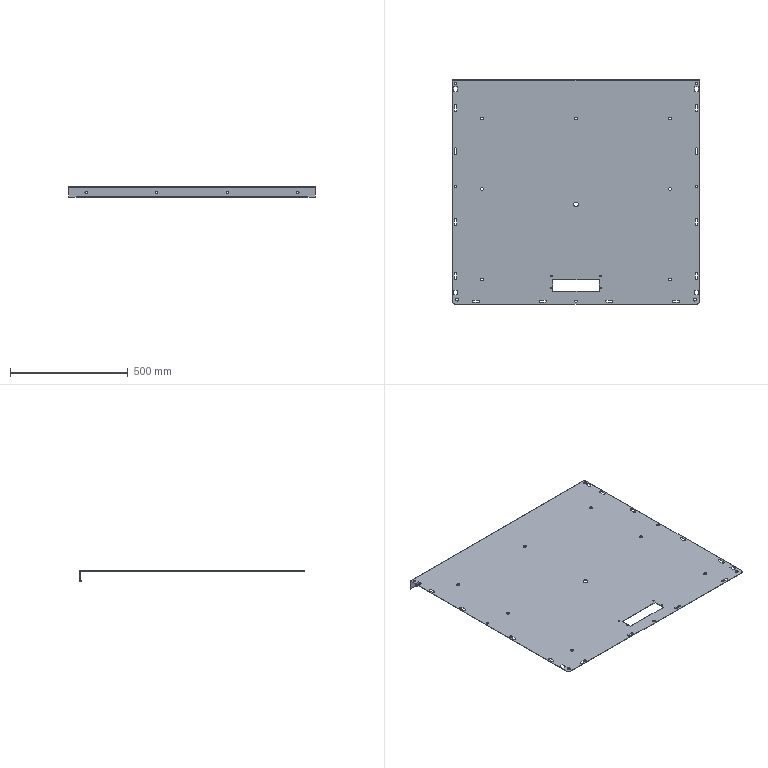Part | 1 solid | 152 faces | box 1050 x 955 x 43.5 mm | volume 1553945 mm3 | cylinder 81 | plane 71 | commonest cylinder face diameters 10 x34 12 x14 6 x8 10.5 x8 11 x5 12.5 x4